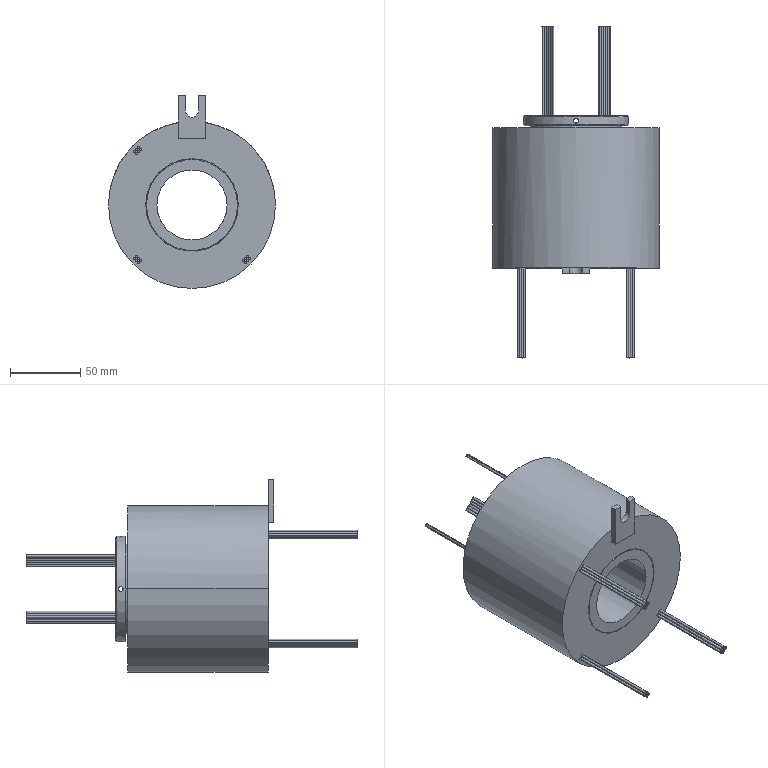Part | SolidWorks | features MBimport 1 | 2 solids | 158 faces | box 119 x 236.5 x 137.5 mm | volume 931913 mm3 | cylinder 95 | plane 51 | cone 12 | commonest cylinder face diameters 1.8 x72 3.4 x8 65 x5 66 x3 50 x2 75 x2